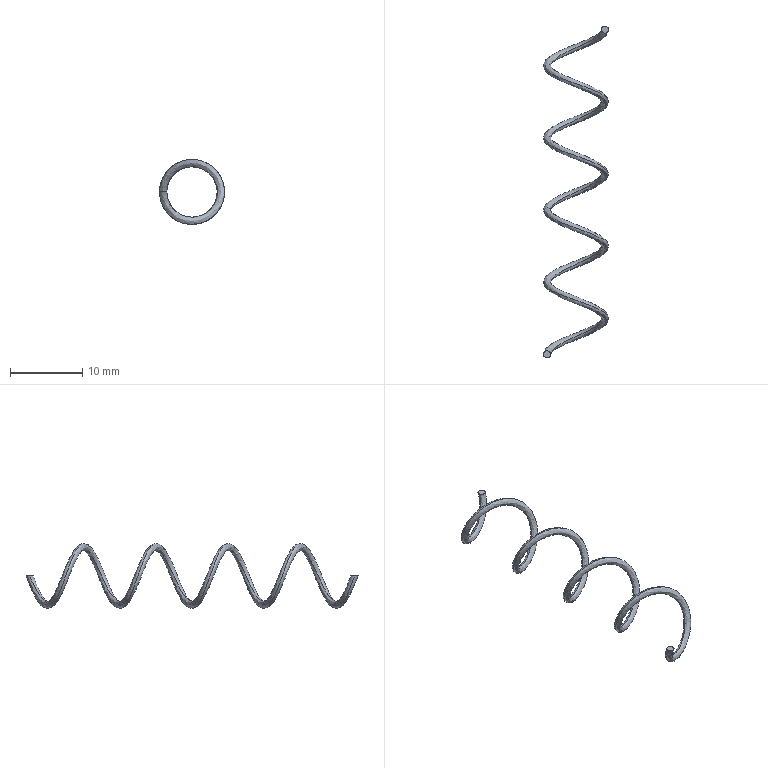Part | SolidWorks | features Helix 1, Sweep 1 | 1 solid | 4 faces | box 9 x 46 x 9 mm | volume 88.855 mm3 | spline 2 | plane 2